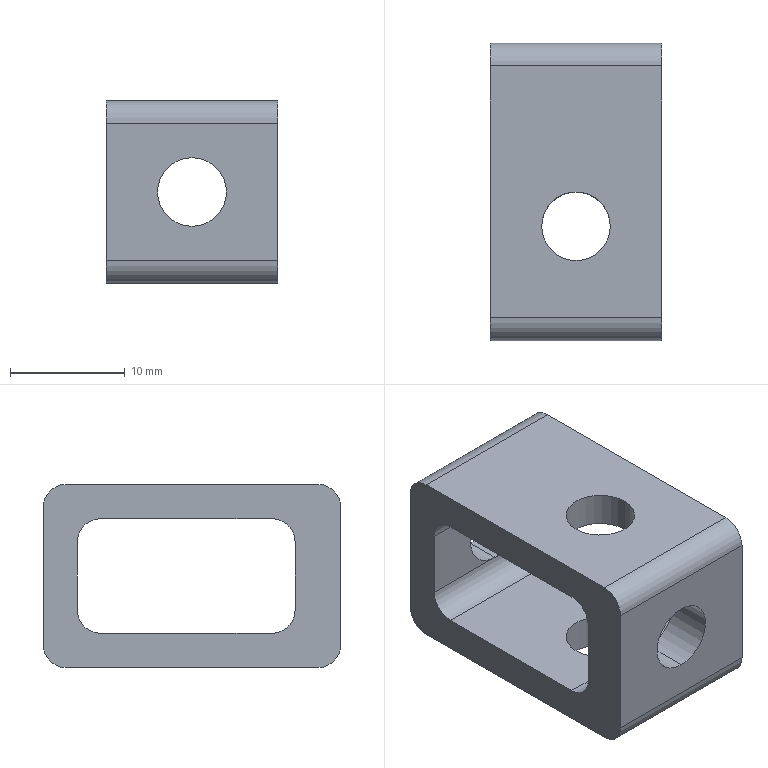Part | SolidWorks | features ICE 3, Fillet 2, Extrusion 1 | 1 solid | 28 faces | box 15 x 26 x 16 mm | volume 3022 mm3 | cylinder 16 | plane 12 | commonest cylinder face diameters 4 x8 6 x8
STEP:
#1=CARTESIAN_POINT('',(0.,-10.,3.));
#2=VERTEX_POINT('',#1);
#3=CARTESIAN_POINT('',(0.,-10.,-3.));
#4=VERTEX_POINT('',#3);
#5=CARTESIAN_POINT('',(0.,-10.,0.));
#6=DIRECTION('',(0.,-1.,0.));
#7=DIRECTION('',(0.,0.,-1.));
#8=AXIS2_PLACEMENT_3D('',#5,#6,#7);
#9=CIRCLE('',#8,3.);
#10=EDGE_CURVE('',#2,#4,#9,.T.);
#11=ORIENTED_EDGE('',*,*,#10,.T.);
#12=CARTESIAN_POINT('',(0.,-6.,-3.));
#13=VERTEX_POINT('',#12);
#14=CARTESIAN_POINT('',(0.,-10.,-3.));
#15=DIRECTION('',(0.,1.,0.));
#16=VECTOR('',#15,1000.);
#17=LINE('',#14,#16);
#18=EDGE_CURVE('',#4,#13,#17,.T.);
#19=ORIENTED_EDGE('',*,*,#18,.T.);
#20=CARTESIAN_POINT('',(0.,-6.,3.));
#21=VERTEX_POINT('',#20);
#22=CARTESIAN_POINT('',(0.,-6.,0.));
#23=DIRECTION('',(0.,-1.,0.));
#24=DIRECTION('',(0.,0.,-1.));
#25=AXIS2_PLACEMENT_3D('',#22,#23,#24);
#26=CIRCLE('',#25,3.);
#27=EDGE_CURVE('',#21,#13,#26,.T.);
#28=ORIENTED_EDGE('',*,*,#27,.F.);
#29=CARTESIAN_POINT('',(0.,-10.,3.));
#30=DIRECTION('',(0.,1.,0.));
#31=VECTOR('',#30,1000.);
#32=LINE('',#29,#31);
#33=EDGE_CURVE('',#2,#21,#32,.T.);
#34=ORIENTED_EDGE('',*,*,#33,.F.);
#35=EDGE_LOOP('',(#11,#19,#28,#34));
#36=FACE_OUTER_BOUND('',#35,.T.);
#37=CARTESIAN_POINT('',(0.,-10.,0.));
#38=DIRECTION('',(0.,1.,0.));
#39=DIRECTION('',(0.,0.,1.));
#40=AXIS2_PLACEMENT_3D('',#37,#38,#39);
#41=CYLINDRICAL_SURFACE('',#40,3.);
#42=ADVANCED_FACE('',(#36),#41,.F.);
#43=CARTESIAN_POINT('',(0.,13.,-3.));
#44=VERTEX_POINT('',#43);
#45=CARTESIAN_POINT('',(0.,13.,3.));
#46=VERTEX_POINT('',#45);
#47=CARTESIAN_POINT('',(0.,13.,0.));
#48=DIRECTION('',(0.,1.,0.));
#49=DIRECTION('',(0.,0.,1.));
#50=AXIS2_PLACEMENT_3D('',#47,#48,#49);
#51=CIRCLE('',#50,3.);
#52=EDGE_CURVE('',#44,#46,#51,.T.);
#53=ORIENTED_EDGE('',*,*,#52,.F.);
#54=CARTESIAN_POINT('',(0.,16.,-3.));
#55=VERTEX_POINT('',#54);
#56=CARTESIAN_POINT('',(0.,-2.,-3.));
#57=DIRECTION('',(0.,1.,0.));
#58=VECTOR('',#57,1000.);
#59=LINE('',#56,#58);
#60=EDGE_CURVE('',#44,#55,#59,.T.);
#61=ORIENTED_EDGE('',*,*,#60,.T.);
#62=CARTESIAN_POINT('',(0.,16.,3.));
#63=VERTEX_POINT('',#62);
#64=CARTESIAN_POINT('',(0.,16.,0.));
#65=DIRECTION('',(0.,1.,0.));
#66=DIRECTION('',(0.,0.,1.));
#67=AXIS2_PLACEMENT_3D('',#64,#65,#66);
#68=CIRCLE('',#67,3.);
#69=EDGE_CURVE('',#55,#63,#68,.T.);
#70=ORIENTED_EDGE('',*,*,#69,.T.);
#71=CARTESIAN_POINT('',(0.,-2.,3.));
#72=DIRECTION('',(0.,1.,0.));
#73=VECTOR('',#72,1000.);
#74=LINE('',#71,#73);
#75=EDGE_CURVE('',#46,#63,#74,.T.);
#76=ORIENTED_EDGE('',*,*,#75,.F.);
#77=EDGE_LOOP('',(#53,#61,#70,#76));
#78=FACE_OUTER_BOUND('',#77,.T.);
#79=CARTESIAN_POINT('',(0.,-2.,0.));
#80=DIRECTION('',(0.,1.,0.));
#81=DIRECTION('',(0.,0.,1.));
#82=AXIS2_PLACEMENT_3D('',#79,#80,#81);
#83=CYLINDRICAL_SURFACE('',#82,3.);
#84=ADVANCED_FACE('',(#78),#83,.F.);
#85=CARTESIAN_POINT('',(3.,0.,-5.));
#86=VERTEX_POINT('',#85);
#87=CARTESIAN_POINT('',(-3.,0.,-5.));
#88=VERTEX_POINT('',#87);
#89=CARTESIAN_POINT('',(0.,0.,-5.));
#90=DIRECTION('',(0.,0.,-1.));
#91=DIRECTION('',(-1.,0.,0.));
#92=AXIS2_PLACEMENT_3D('',#89,#90,#91);
#93=CIRCLE('',#92,3.);
#94=EDGE_CURVE('',#86,#88,#93,.T.);
#95=ORIENTED_EDGE('',*,*,#94,.F.);
#96=CARTESIAN_POINT('',(3.,0.,-8.));
#97=VERTEX_POINT('',#96);
#98=CARTESIAN_POINT('',(3.,0.,8.));
#99=DIRECTION('',(0.,0.,-1.));
#100=VECTOR('',#99,1000.);
#101=LINE('',#98,#100);
#102=EDGE_CURVE('',#86,#97,#101,.T.);
#103=ORIENTED_EDGE('',*,*,#102,.T.);
#104=CARTESIAN_POINT('',(-3.,0.,-8.));
#105=VERTEX_POINT('',#104);
#106=CARTESIAN_POINT('',(0.,0.,-8.));
#107=DIRECTION('',(0.,0.,1.));
#108=DIRECTION('',(1.,0.,0.));
#109=AXIS2_PLACEMENT_3D('',#106,#107,#108);
#110=CIRCLE('',#109,3.);
#111=EDGE_CURVE('',#105,#97,#110,.T.);
#112=ORIENTED_EDGE('',*,*,#111,.F.);
#113=CARTESIAN_POINT('',(-3.,0.,8.));
#114=DIRECTION('',(0.,0.,-1.));
#115=VECTOR('',#114,1000.);
#116=LINE('',#113,#115);
#117=EDGE_CURVE('',#88,#105,#116,.T.);
#118=ORIENTED_EDGE('',*,*,#117,.F.);
#119=EDGE_LOOP('',(#95,#103,#112,#118));
#120=FACE_OUTER_BOUND('',#119,.T.);
#121=CARTESIAN_POINT('',(0.,0.,8.));
#122=DIRECTION('',(0.,0.,-1.));
#123=DIRECTION('',(-1.,0.,0.));
#124=AXIS2_PLACEMENT_3D('',#121,#122,#123);
#125=CYLINDRICAL_SURFACE('',#124,3.);
#126=ADVANCED_FACE('',(#120),#125,.F.);
#127=CARTESIAN_POINT('',(-3.,0.,8.));
#128=VERTEX_POINT('',#127);
#129=CARTESIAN_POINT('',(3.,0.,8.));
#130=VERTEX_POINT('',#129);
#131=CARTESIAN_POINT('',(0.,0.,8.));
#132=DIRECTION('',(0.,0.,1.));
#133=DIRECTION('',(1.,0.,0.));
#134=AXIS2_PLACEMENT_3D('',#131,#132,#133);
#135=CIRCLE('',#134,3.);
#136=EDGE_CURVE('',#128,#130,#135,.T.);
#137=ORIENTED_EDGE('',*,*,#136,.T.);
#138=CARTESIAN_POINT('',(3.,0.,5.));
#139=VERTEX_POINT('',#138);
#140=CARTESIAN_POINT('',(3.,0.,8.));
#141=DIRECTION('',(0.,0.,-1.));
#142=VECTOR('',#141,1000.);
#143=LINE('',#140,#142);
#144=EDGE_CURVE('',#130,#139,#143,.T.);
#145=ORIENTED_EDGE('',*,*,#144,.T.);
#146=CARTESIAN_POINT('',(-3.,0.,5.));
#147=VERTEX_POINT('',#146);
#148=CARTESIAN_POINT('',(0.,0.,5.));
#149=DIRECTION('',(0.,0.,1.));
#150=DIRECTION('',(1.,0.,0.));
#151=AXIS2_PLACEMENT_3D('',#148,#149,#150);
#152=CIRCLE('',#151,3.);
#153=EDGE_CURVE('',#147,#139,#152,.T.);
#154=ORIENTED_EDGE('',*,*,#153,.F.);
#155=CARTESIAN_POINT('',(-3.,0.,8.));
#156=DIRECTION('',(0.,0.,-1.));
#157=VECTOR('',#156,1000.);
#158=LINE('',#155,#157);
#159=EDGE_CURVE('',#128,#147,#158,.T.);
#160=ORIENTED_EDGE('',*,*,#159,.F.);
#161=EDGE_LOOP('',(#137,#145,#154,#160));
#162=FACE_OUTER_BOUND('',#161,.T.);
#163=CARTESIAN_POINT('',(0.,0.,8.));
#164=DIRECTION('',(0.,0.,-1.));
#165=DIRECTION('',(-1.,0.,0.));
#166=AXIS2_PLACEMENT_3D('',#163,#164,#165);
#167=CYLINDRICAL_SURFACE('',#166,3.);
#168=ADVANCED_FACE('',(#162),#167,.F.);
#169=CARTESIAN_POINT('',(7.5,-6.,-3.));
#170=VERTEX_POINT('',#169);
#171=CARTESIAN_POINT('',(7.5,-6.,3.));
#172=VERTEX_POINT('',#171);
#173=CARTESIAN_POINT('',(7.5,-6.,-8.));
#174=DIRECTION('',(0.,0.,1.));
#175=VECTOR('',#174,1000.);
#176=LINE('',#173,#175);
#177=EDGE_CURVE('',#170,#172,#176,.T.);
#178=ORIENTED_EDGE('',*,*,#177,.F.);
#179=CARTESIAN_POINT('',(0.,-6.,-3.));
#180=DIRECTION('',(-1.,0.,0.));
#181=VECTOR('',#180,1000.);
#182=LINE('',#179,#181);
#183=EDGE_CURVE('',#170,#13,#182,.T.);
#184=ORIENTED_EDGE('',*,*,#183,.T.);
#185=CARTESIAN_POINT('',(0.,-6.,0.));
#186=DIRECTION('',(0.,-1.,0.));
#187=DIRECTION('',(0.,0.,-1.));
#188=AXIS2_PLACEMENT_3D('',#185,#186,#187);
#189=CIRCLE('',#188,3.);
#190=EDGE_CURVE('',#13,#21,#189,.T.);
#191=ORIENTED_EDGE('',*,*,#190,.T.);
#192=CARTESIAN_POINT('',(0.,-6.,3.));
#193=DIRECTION('',(1.,0.,0.));
#194=VECTOR('',#193,1000.);
#195=LINE('',#192,#194);
#196=EDGE_CURVE('',#21,#172,#195,.T.);
#197=ORIENTED_EDGE('',*,*,#196,.T.);
#198=EDGE_LOOP('',(#178,#184,#191,#197));
#199=FACE_OUTER_BOUND('',#198,.T.);
#200=CARTESIAN_POINT('',(0.,-6.,0.));
#201=DIRECTION('',(0.,1.,0.));
#202=DIRECTION('',(0.,0.,1.));
#203=AXIS2_PLACEMENT_3D('',#200,#201,#202);
#204=PLANE('',#203);
#205=ADVANCED_FACE('',(#199),#204,.T.);
#206=CARTESIAN_POINT('',(7.5,13.,3.));
#207=VERTEX_POINT('',#206);
#208=CARTESIAN_POINT('',(-7.5,13.,3.));
#209=DIRECTION('',(-1.,0.,0.));
#210=VECTOR('',#209,1000.);
#211=LINE('',#208,#210);
#212=EDGE_CURVE('',#207,#46,#211,.T.);
#213=ORIENTED_EDGE('',*,*,#212,.T.);
#214=CARTESIAN_POINT('',(0.,13.,0.));
#215=DIRECTION('',(0.,1.,0.));
#216=DIRECTION('',(0.,0.,1.));
#217=AXIS2_PLACEMENT_3D('',#214,#215,#216);
#218=CIRCLE('',#217,3.);
#219=EDGE_CURVE('',#46,#44,#218,.T.);
#220=ORIENTED_EDGE('',*,*,#219,.T.);
#221=CARTESIAN_POINT('',(7.5,13.,-3.));
#222=VERTEX_POINT('',#221);
#223=CARTESIAN_POINT('',(7.5,13.,-3.));
#224=DIRECTION('',(1.,0.,0.));
#225=VECTOR('',#224,1000.);
#226=LINE('',#223,#225);
#227=EDGE_CURVE('',#44,#222,#226,.T.);
#228=ORIENTED_EDGE('',*,*,#227,.T.);
#229=CARTESIAN_POINT('',(7.5,13.,5.));
#230=DIRECTION('',(0.,0.,1.));
#231=VECTOR('',#230,1000.);
#232=LINE('',#229,#231);
#233=EDGE_CURVE('',#222,#207,#232,.T.);
#234=ORIENTED_EDGE('',*,*,#233,.T.);
#235=EDGE_LOOP('',(#213,#220,#228,#234));
#236=FACE_OUTER_BOUND('',#235,.T.);
#237=CARTESIAN_POINT('',(-7.5,13.,5.));
#238=DIRECTION('',(0.,1.,0.));
#239=DIRECTION('',(0.,0.,1.));
#240=AXIS2_PLACEMENT_3D('',#237,#238,#239);
#241=PLANE('',#240);
#242=ADVANCED_FACE('',(#236),#241,.F.);
#243=ORIENTED_EDGE('',*,*,#144,.F.);
#244=CARTESIAN_POINT('',(0.,0.,8.));
#245=DIRECTION('',(0.,0.,1.));
#246=DIRECTION('',(1.,0.,0.));
#247=AXIS2_PLACEMENT_3D('',#244,#245,#246);
#248=CIRCLE('',#247,3.);
#249=EDGE_CURVE('',#130,#128,#248,.T.);
#250=ORIENTED_EDGE('',*,*,#249,.T.);
#251=ORIENTED_EDGE('',*,*,#159,.T.);
#252=CARTESIAN_POINT('',(0.,0.,5.));
#253=DIRECTION('',(0.,0.,1.));
#254=DIRECTION('',(1.,0.,0.));
#255=AXIS2_PLACEMENT_3D('',#252,#253,#254);
#256=CIRCLE('',#255,3.);
#257=EDGE_CURVE('',#139,#147,#256,.T.);
#258=ORIENTED_EDGE('',*,*,#257,.F.);
#259=EDGE_LOOP('',(#243,#250,#251,#258));
#260=FACE_OUTER_BOUND('',#259,.T.);
#261=CARTESIAN_POINT('',(0.,0.,8.));
#262=DIRECTION('',(0.,0.,-1.));
#263=DIRECTION('',(-1.,0.,0.));
#264=AXIS2_PLACEMENT_3D('',#261,#262,#263);
#265=CYLINDRICAL_SURFACE('',#264,3.);
#266=ADVANCED_FACE('',(#260),#265,.F.);
#267=CARTESIAN_POINT('',(-7.5,14.,8.));
#268=VERTEX_POINT('',#267);
#269=CARTESIAN_POINT('',(-7.5,-8.,8.));
#270=VERTEX_POINT('',#269);
#271=CARTESIAN_POINT('',(-7.5,-6.,8.));
#272=DIRECTION('',(0.,-1.,0.));
#273=VECTOR('',#272,1000.);
#274=LINE('',#271,#273);
#275=EDGE_CURVE('',#268,#270,#274,.T.);
#276=ORIENTED_EDGE('',*,*,#275,.T.);
#277=CARTESIAN_POINT('',(7.5,-8.,8.));
#278=VERTEX_POINT('',#277);
#279=CARTESIAN_POINT('',(0.,-8.,8.));
#280=DIRECTION('',(1.,0.,0.));
#281=VECTOR('',#280,1000.);
#282=LINE('',#279,#281);
#283=EDGE_CURVE('',#270,#278,#282,.T.);
#284=ORIENTED_EDGE('',*,*,#283,.T.);
#285=CARTESIAN_POINT('',(7.5,14.,8.));
#286=VERTEX_POINT('',#285);
#287=CARTESIAN_POINT('',(7.5,-6.,8.));
#288=DIRECTION('',(0.,1.,0.));
#289=VECTOR('',#288,1000.);
#290=LINE('',#287,#289);
#291=EDGE_CURVE('',#278,#286,#290,.T.);
#292=ORIENTED_EDGE('',*,*,#291,.T.);
#293=CARTESIAN_POINT('',(0.,14.,8.));
#294=DIRECTION('',(-1.,0.,0.));
#295=VECTOR('',#294,1000.);
#296=LINE('',#293,#295);
#297=EDGE_CURVE('',#286,#268,#296,.T.);
#298=ORIENTED_EDGE('',*,*,#297,.T.);
#299=EDGE_LOOP('',(#276,#284,#292,#298));
#300=FACE_OUTER_BOUND('',#299,.T.);
#301=ORIENTED_EDGE('',*,*,#136,.F.);
#302=ORIENTED_EDGE('',*,*,#249,.F.);
#303=EDGE_LOOP('',(#301,#302));
#304=FACE_BOUND('',#303,.T.);
#305=CARTESIAN_POINT('',(0.,0.,8.));
#306=DIRECTION('',(0.,0.,-1.));
#307=DIRECTION('',(-1.,0.,0.));
#308=AXIS2_PLACEMENT_3D('',#305,#306,#307);
#309=PLANE('',#308);
#310=ADVANCED_FACE('',(#300,#304),#309,.F.);
#311=CARTESIAN_POINT('',(7.5,-8.,-8.));
#312=VERTEX_POINT('',#311);
#313=CARTESIAN_POINT('',(7.5,14.,-8.));
#314=VERTEX_POINT('',#313);
#315=CARTESIAN_POINT('',(7.5,-6.,-8.));
#316=DIRECTION('',(0.,1.,0.));
#317=VECTOR('',#316,1000.);
#318=LINE('',#315,#317);
#319=EDGE_CURVE('',#312,#314,#318,.T.);
#320=ORIENTED_EDGE('',*,*,#319,.F.);
#321=CARTESIAN_POINT('',(-7.5,-8.,-8.));
#322=VERTEX_POINT('',#321);
#323=CARTESIAN_POINT('',(-7.5,-8.,-8.));
#324=DIRECTION('',(-1.,0.,0.));
#325=VECTOR('',#324,1000.);
#326=LINE('',#323,#325);
#327=EDGE_CURVE('',#312,#322,#326,.T.);
#328=ORIENTED_EDGE('',*,*,#327,.T.);
#329=CARTESIAN_POINT('',(-7.5,14.,-8.));
#330=VERTEX_POINT('',#329);
#331=CARTESIAN_POINT('',(-7.5,-6.,-8.));
#332=DIRECTION('',(0.,-1.,0.));
#333=VECTOR('',#332,1000.);
#334=LINE('',#331,#333);
#335=EDGE_CURVE('',#330,#322,#334,.T.);
#336=ORIENTED_EDGE('',*,*,#335,.F.);
#337=CARTESIAN_POINT('',(7.5,14.,-8.));
#338=DIRECTION('',(1.,0.,0.));
#339=VECTOR('',#338,1000.);
#340=LINE('',#337,#339);
#341=EDGE_CURVE('',#330,#314,#340,.T.);
#342=ORIENTED_EDGE('',*,*,#341,.T.);
#343=EDGE_LOOP('',(#320,#328,#336,#342));
#344=FACE_OUTER_BOUND('',#343,.T.);
#345=ORIENTED_EDGE('',*,*,#111,.T.);
#346=CARTESIAN_POINT('',(0.,0.,-8.));
#347=DIRECTION('',(0.,0.,1.));
#348=DIRECTION('',(1.,0.,0.));
#349=AXIS2_PLACEMENT_3D('',#346,#347,#348);
#350=CIRCLE('',#349,3.);
#351=EDGE_CURVE('',#97,#105,#350,.T.);
#352=ORIENTED_EDGE('',*,*,#351,.T.);
#353=EDGE_LOOP('',(#345,#352));
#354=FACE_BOUND('',#353,.T.);
#355=CARTESIAN_POINT('',(0.,0.,-8.));
#356=DIRECTION('',(0.,0.,-1.));
#357=DIRECTION('',(-1.,0.,0.));
#358=AXIS2_PLACEMENT_3D('',#355,#356,#357);
#359=PLANE('',#358);
#360=ADVANCED_FACE('',(#344,#354),#359,.T.);
#361=CARTESIAN_POINT('',(-7.5,11.,5.));
#362=VERTEX_POINT('',#361);
#363=CARTESIAN_POINT('',(-7.5,-4.,5.));
#364=VERTEX_POINT('',#363);
#365=CARTESIAN_POINT('',(-7.5,-6.,5.));
#366=DIRECTION('',(0.,-1.,0.));
#367=VECTOR('',#366,1000.);
#368=LINE('',#365,#367);
#369=EDGE_CURVE('',#362,#364,#368,.T.);
#370=ORIENTED_EDGE('',*,*,#369,.T.);
#371=CARTESIAN_POINT('',(-7.5,-6.,3.));
#372=VERTEX_POINT('',#371);
#373=CARTESIAN_POINT('',(-7.5,-4.,3.));
#374=DIRECTION('',(1.,0.,0.));
#375=DIRECTION('',(0.,0.,-1.));
#376=AXIS2_PLACEMENT_3D('',#373,#374,#375);
#377=CIRCLE('',#376,2.);
#378=EDGE_CURVE('',#364,#372,#377,.T.);
#379=ORIENTED_EDGE('',*,*,#378,.T.);
#380=CARTESIAN_POINT('',(-7.5,-6.,-3.));
#381=VERTEX_POINT('',#380);
#382=CARTESIAN_POINT('',(-7.5,-6.,-8.));
#383=DIRECTION('',(0.,0.,-1.));
#384=VECTOR('',#383,1000.);
#385=LINE('',#382,#384);
#386=EDGE_CURVE('',#372,#381,#385,.T.);
#387=ORIENTED_EDGE('',*,*,#386,.T.);
#388=CARTESIAN_POINT('',(-7.5,-4.,-5.));
#389=VERTEX_POINT('',#388);
#390=CARTESIAN_POINT('',(-7.5,-4.,-3.));
#391=DIRECTION('',(1.,0.,0.));
#392=DIRECTION('',(0.,0.,-1.));
#393=AXIS2_PLACEMENT_3D('',#390,#391,#392);
#394=CIRCLE('',#393,2.);
#395=EDGE_CURVE('',#381,#389,#394,.T.);
#396=ORIENTED_EDGE('',*,*,#395,.T.);
#397=CARTESIAN_POINT('',(-7.5,11.,-5.));
#398=VERTEX_POINT('',#397);
#399=CARTESIAN_POINT('',(-7.5,-6.,-5.));
#400=DIRECTION('',(0.,1.,0.));
#401=VECTOR('',#400,1000.);
#402=LINE('',#399,#401);
#403=EDGE_CURVE('',#389,#398,#402,.T.);
#404=ORIENTED_EDGE('',*,*,#403,.T.);
#405=CARTESIAN_POINT('',(-7.5,13.,-3.));
#406=VERTEX_POINT('',#405);
#407=CARTESIAN_POINT('',(-7.5,11.,-3.));
#408=DIRECTION('',(1.,0.,0.));
#409=DIRECTION('',(0.,0.,-1.));
#410=AXIS2_PLACEMENT_3D('',#407,#408,#409);
#411=CIRCLE('',#410,2.);
#412=EDGE_CURVE('',#398,#406,#411,.T.);
#413=ORIENTED_EDGE('',*,*,#412,.T.);
#414=CARTESIAN_POINT('',(-7.5,13.,3.));
#415=VERTEX_POINT('',#414);
#416=CARTESIAN_POINT('',(-7.5,13.,5.));
#417=DIRECTION('',(0.,0.,1.));
#418=VECTOR('',#417,1000.);
#419=LINE('',#416,#418);
#420=EDGE_CURVE('',#406,#415,#419,.T.);
#421=ORIENTED_EDGE('',*,*,#420,.T.);
#422=CARTESIAN_POINT('',(-7.5,11.,3.));
#423=DIRECTION('',(1.,0.,0.));
#424=DIRECTION('',(0.,0.,-1.));
#425=AXIS2_PLACEMENT_3D('',#422,#423,#424);
#426=CIRCLE('',#425,2.);
#427=EDGE_CURVE('',#415,#362,#426,.T.);
#428=ORIENTED_EDGE('',*,*,#427,.T.);
#429=EDGE_LOOP('',(#370,#379,#387,#396,#404,#413,#421,#428));
#430=FACE_BOUND('',#429,.T.);
#431=ORIENTED_EDGE('',*,*,#335,.T.);
#432=CARTESIAN_POINT('',(-7.5,-10.,-6.));
#433=VERTEX_POINT('',#432);
#434=CARTESIAN_POINT('',(-7.5,-8.,-6.));
#435=DIRECTION('',(-1.,0.,0.));
#436=DIRECTION('',(0.,0.,-1.));
#437=AXIS2_PLACEMENT_3D('',#434,#435,#436);
#438=CIRCLE('',#437,2.);
#439=EDGE_CURVE('',#322,#433,#438,.T.);
#440=ORIENTED_EDGE('',*,*,#439,.T.);
#441=CARTESIAN_POINT('',(-7.5,-10.,6.));
#442=VERTEX_POINT('',#441);
#443=CARTESIAN_POINT('',(-7.5,-10.,-8.));
#444=DIRECTION('',(0.,0.,-1.));
#445=VECTOR('',#444,1000.);
#446=LINE('',#443,#445);
#447=EDGE_CURVE('',#442,#433,#446,.T.);
#448=ORIENTED_EDGE('',*,*,#447,.F.);
#449=CARTESIAN_POINT('',(-7.5,-8.,6.));
#450=DIRECTION('',(-1.,0.,0.));
#451=DIRECTION('',(0.,0.,-1.));
#452=AXIS2_PLACEMENT_3D('',#449,#450,#451);
#453=CIRCLE('',#452,2.);
#454=EDGE_CURVE('',#442,#270,#453,.T.);
#455=ORIENTED_EDGE('',*,*,#454,.T.);
#456=ORIENTED_EDGE('',*,*,#275,.F.);
#457=CARTESIAN_POINT('',(-7.5,16.,6.));
#458=VERTEX_POINT('',#457);
#459=CARTESIAN_POINT('',(-7.5,14.,6.));
#460=DIRECTION('',(-1.,0.,0.));
#461=DIRECTION('',(0.,0.,-1.));
#462=AXIS2_PLACEMENT_3D('',#459,#460,#461);
#463=CIRCLE('',#462,2.);
#464=EDGE_CURVE('',#268,#458,#463,.T.);
#465=ORIENTED_EDGE('',*,*,#464,.T.);
#466=CARTESIAN_POINT('',(-7.5,16.,-6.));
#467=VERTEX_POINT('',#466);
#468=CARTESIAN_POINT('',(-7.5,16.,8.));
#469=DIRECTION('',(0.,0.,-1.));
#470=VECTOR('',#469,1000.);
#471=LINE('',#468,#470);
#472=EDGE_CURVE('',#458,#467,#471,.T.);
#473=ORIENTED_EDGE('',*,*,#472,.T.);
#474=CARTESIAN_POINT('',(-7.5,14.,-6.));
#475=DIRECTION('',(-1.,0.,0.));
#476=DIRECTION('',(0.,0.,-1.));
#477=AXIS2_PLACEMENT_3D('',#474,#475,#476);
#478=CIRCLE('',#477,2.);
#479=EDGE_CURVE('',#467,#330,#478,.T.);
#480=ORIENTED_EDGE('',*,*,#479,.T.);
#481=EDGE_LOOP('',(#431,#440,#448,#455,#456,#465,#473,#480));
#482=FACE_OUTER_BOUND('',#481,.T.);
#483=CARTESIAN_POINT('',(-7.5,-6.,8.));
#484=DIRECTION('',(1.,0.,0.));
#485=DIRECTION('',(0.,0.,-1.));
#486=AXIS2_PLACEMENT_3D('',#483,#484,#485);
#487=PLANE('',#486);
#488=ADVANCED_FACE('',(#430,#482),#487,.F.);
#489=CARTESIAN_POINT('',(7.5,-4.,-5.));
#490=VERTEX_POINT('',#489);
#491=CARTESIAN_POINT('',(7.5,11.,-5.));
#492=VERTEX_POINT('',#491);
#493=CARTESIAN_POINT('',(7.5,-6.,-5.));
#494=DIRECTION('',(0.,1.,0.));
#495=VECTOR('',#494,1000.);
#496=LINE('',#493,#495);
#497=EDGE_CURVE('',#490,#492,#496,.T.);
#498=ORIENTED_EDGE('',*,*,#497,.F.);
#499=CARTESIAN_POINT('',(7.5,-4.,-3.));
#500=DIRECTION('',(-1.,0.,0.));
#501=DIRECTION('',(0.,0.,1.));
#502=AXIS2_PLACEMENT_3D('',#499,#500,#501);
#503=CIRCLE('',#502,2.);
#504=EDGE_CURVE('',#490,#170,#503,.T.);
#505=ORIENTED_EDGE('',*,*,#504,.T.);
#506=ORIENTED_EDGE('',*,*,#177,.T.);
#507=CARTESIAN_POINT('',(7.5,-4.,5.));
#508=VERTEX_POINT('',#507);
#509=CARTESIAN_POINT('',(7.5,-4.,3.));
#510=DIRECTION('',(-1.,0.,0.));
#511=DIRECTION('',(0.,0.,1.));
#512=AXIS2_PLACEMENT_3D('',#509,#510,#511);
#513=CIRCLE('',#512,2.);
#514=EDGE_CURVE('',#172,#508,#513,.T.);
#515=ORIENTED_EDGE('',*,*,#514,.T.);
#516=CARTESIAN_POINT('',(7.5,11.,5.));
#517=VERTEX_POINT('',#516);
#518=CARTESIAN_POINT('',(7.5,-6.,5.));
#519=DIRECTION('',(0.,-1.,0.));
#520=VECTOR('',#519,1000.);
#521=LINE('',#518,#520);
#522=EDGE_CURVE('',#517,#508,#521,.T.);
#523=ORIENTED_EDGE('',*,*,#522,.F.);
#524=CARTESIAN_POINT('',(7.5,11.,3.));
#525=DIRECTION('',(-1.,0.,0.));
#526=DIRECTION('',(0.,0.,1.));
#527=AXIS2_PLACEMENT_3D('',#524,#525,#526);
#528=CIRCLE('',#527,2.);
#529=EDGE_CURVE('',#517,#207,#528,.T.);
#530=ORIENTED_EDGE('',*,*,#529,.T.);
#531=ORIENTED_EDGE('',*,*,#233,.F.);
#532=CARTESIAN_POINT('',(7.5,11.,-3.));
#533=DIRECTION('',(-1.,0.,0.));
#534=DIRECTION('',(0.,0.,1.));
#535=AXIS2_PLACEMENT_3D('',#532,#533,#534);
#536=CIRCLE('',#535,2.);
#537=EDGE_CURVE('',#222,#492,#536,.T.);
#538=ORIENTED_EDGE('',*,*,#537,.T.);
#539=EDGE_LOOP('',(#498,#505,#506,#515,#523,#530,#531,#538));
#540=FACE_BOUND('',#539,.T.);
#541=CARTESIAN_POINT('',(7.5,-10.,-6.));
#542=VERTEX_POINT('',#541);
#543=CARTESIAN_POINT('',(7.5,-10.,6.));
#544=VERTEX_POINT('',#543);
#545=CARTESIAN_POINT('',(7.5,-10.,-8.));
#546=DIRECTION('',(0.,0.,1.));
#547=VECTOR('',#546,1000.);
#548=LINE('',#545,#547);
#549=EDGE_CURVE('',#542,#544,#548,.T.);
#550=ORIENTED_EDGE('',*,*,#549,.F.);
#551=CARTESIAN_POINT('',(7.5,-8.,-6.));
#552=DIRECTION('',(1.,0.,0.));
#553=DIRECTION('',(0.,0.,1.));
#554=AXIS2_PLACEMENT_3D('',#551,#552,#553);
#555=CIRCLE('',#554,2.);
#556=EDGE_CURVE('',#542,#312,#555,.T.);
#557=ORIENTED_EDGE('',*,*,#556,.T.);
#558=ORIENTED_EDGE('',*,*,#319,.T.);
#559=CARTESIAN_POINT('',(7.5,16.,-6.));
#560=VERTEX_POINT('',#559);
#561=CARTESIAN_POINT('',(7.5,14.,-6.));
#562=DIRECTION('',(1.,0.,0.));
#563=DIRECTION('',(0.,0.,1.));
#564=AXIS2_PLACEMENT_3D('',#561,#562,#563);
#565=CIRCLE('',#564,2.);
#566=EDGE_CURVE('',#314,#560,#565,.T.);
#567=ORIENTED_EDGE('',*,*,#566,.T.);
#568=CARTESIAN_POINT('',(7.5,16.,6.));
#569=VERTEX_POINT('',#568);
#570=CARTESIAN_POINT('',(7.5,16.,8.));
#571=DIRECTION('',(0.,0.,-1.));
#572=VECTOR('',#571,1000.);
#573=LINE('',#570,#572);
#574=EDGE_CURVE('',#569,#560,#573,.T.);
#575=ORIENTED_EDGE('',*,*,#574,.F.);
#576=CARTESIAN_POINT('',(7.5,14.,6.));
#577=DIRECTION('',(1.,0.,0.));
#578=DIRECTION('',(0.,0.,1.));
#579=AXIS2_PLACEMENT_3D('',#576,#577,#578);
#580=CIRCLE('',#579,2.);
#581=EDGE_CURVE('',#569,#286,#580,.T.);
#582=ORIENTED_EDGE('',*,*,#581,.T.);
#583=ORIENTED_EDGE('',*,*,#291,.F.);
#584=CARTESIAN_POINT('',(7.5,-8.,6.));
#585=DIRECTION('',(1.,0.,0.));
#586=DIRECTION('',(0.,0.,1.));
#587=AXIS2_PLACEMENT_3D('',#584,#585,#586);
#588=CIRCLE('',#587,2.);
#589=EDGE_CURVE('',#278,#544,#588,.T.);
#590=ORIENTED_EDGE('',*,*,#589,.T.);
#591=EDGE_LOOP('',(#550,#557,#558,#567,#575,#582,#583,#590));
#592=FACE_OUTER_BOUND('',#591,.T.);
#593=CARTESIAN_POINT('',(7.5,-6.,8.));
#594=DIRECTION('',(-1.,0.,0.));
#595=DIRECTION('',(0.,0.,1.));
#596=AXIS2_PLACEMENT_3D('',#593,#594,#595);
#597=PLANE('',#596);
#598=ADVANCED_FACE('',(#540,#592),#597,.F.);
#599=CARTESIAN_POINT('',(0.,16.,0.));
#600=DIRECTION('',(0.,1.,0.));
#601=DIRECTION('',(0.,0.,1.));
#602=AXIS2_PLACEMENT_3D('',#599,#600,#601);
#603=CIRCLE('',#602,3.);
#604=EDGE_CURVE('',#63,#55,#603,.T.);
#605=ORIENTED_EDGE('',*,*,#604,.F.);
#606=ORIENTED_EDGE('',*,*,#69,.F.);
#607=EDGE_LOOP('',(#605,#606));
#608=FACE_BOUND('',#607,.T.);
#609=ORIENTED_EDGE('',*,*,#574,.T.);
#610=CARTESIAN_POINT('',(-7.5,16.,-6.));
#611=DIRECTION('',(-1.,0.,0.));
#612=VECTOR('',#611,1000.);
#613=LINE('',#610,#612);
#614=EDGE_CURVE('',#560,#467,#613,.T.);
#615=ORIENTED_EDGE('',*,*,#614,.T.);
#616=ORIENTED_EDGE('',*,*,#472,.F.);
#617=CARTESIAN_POINT('',(-7.5,16.,6.));
#618=DIRECTION('',(1.,0.,0.));
#619=VECTOR('',#618,1000.);
#620=LINE('',#617,#619);
#621=EDGE_CURVE('',#458,#569,#620,.T.);
#622=ORIENTED_EDGE('',*,*,#621,.T.);
#623=EDGE_LOOP('',(#609,#615,#616,#622));
#624=FACE_OUTER_BOUND('',#623,.T.);
#625=CARTESIAN_POINT('',(-7.5,16.,8.));
#626=DIRECTION('',(0.,-1.,0.));
#627=DIRECTION('',(0.,0.,-1.));
#628=AXIS2_PLACEMENT_3D('',#625,#626,#627);
#629=PLANE('',#628);
#630=ADVANCED_FACE('',(#608,#624),#629,.F.);
#631=ORIENTED_EDGE('',*,*,#102,.F.);
#632=CARTESIAN_POINT('',(0.,0.,-5.));
#633=DIRECTION('',(0.,0.,-1.));
#634=DIRECTION('',(-1.,0.,0.));
#635=AXIS2_PLACEMENT_3D('',#632,#633,#634);
#636=CIRCLE('',#635,3.);
#637=EDGE_CURVE('',#88,#86,#636,.T.);
#638=ORIENTED_EDGE('',*,*,#637,.F.);
#639=ORIENTED_EDGE('',*,*,#117,.T.);
#640=ORIENTED_EDGE('',*,*,#351,.F.);
#641=EDGE_LOOP('',(#631,#638,#639,#640));
#642=FACE_OUTER_BOUND('',#641,.T.);
#643=CARTESIAN_POINT('',(0.,0.,8.));
#644=DIRECTION('',(0.,0.,-1.));
#645=DIRECTION('',(-1.,0.,0.));
#646=AXIS2_PLACEMENT_3D('',#643,#644,#645);
#647=CYLINDRICAL_SURFACE('',#646,3.);
#648=ADVANCED_FACE('',(#642),#647,.F.);
#649=ORIENTED_EDGE('',*,*,#153,.T.);
#650=ORIENTED_EDGE('',*,*,#257,.T.);
#651=EDGE_LOOP('',(#649,#650));
#652=FACE_BOUND('',#651,.T.);
#653=ORIENTED_EDGE('',*,*,#522,.T.);
#654=CARTESIAN_POINT('',(-7.5,-4.,5.));
#655=DIRECTION('',(-1.,0.,0.));
#656=VECTOR('',#655,1000.);
#657=LINE('',#654,#656);
#658=EDGE_CURVE('',#508,#364,#657,.T.);
#659=ORIENTED_EDGE('',*,*,#658,.T.);
#660=ORIENTED_EDGE('',*,*,#369,.F.);
#661=CARTESIAN_POINT('',(7.5,11.,5.));
#662=DIRECTION('',(1.,0.,0.));
#663=VECTOR('',#662,1000.);
#664=LINE('',#661,#663);
#665=EDGE_CURVE('',#362,#517,#664,.T.);
#666=ORIENTED_EDGE('',*,*,#665,.T.);
#667=EDGE_LOOP('',(#653,#659,#660,#666));
#668=FACE_OUTER_BOUND('',#667,.T.);
#669=CARTESIAN_POINT('',(-7.5,-6.,5.));
#670=DIRECTION('',(0.,0.,1.));
#671=DIRECTION('',(1.,0.,0.));
#672=AXIS2_PLACEMENT_3D('',#669,#670,#671);
#673=PLANE('',#672);
#674=ADVANCED_FACE('',(#652,#668),#673,.F.);
#675=CARTESIAN_POINT('',(7.5,13.,-3.));
#676=DIRECTION('',(1.,0.,0.));
#677=VECTOR('',#676,1000.);
#678=LINE('',#675,#677);
#679=EDGE_CURVE('',#406,#44,#678,.T.);
#680=ORIENTED_EDGE('',*,*,#679,.T.);
#681=ORIENTED_EDGE('',*,*,#52,.T.);
#682=CARTESIAN_POINT('',(-7.5,13.,3.));
#683=DIRECTION('',(-1.,0.,0.));
#684=VECTOR('',#683,1000.);
#685=LINE('',#682,#684);
#686=EDGE_CURVE('',#46,#415,#685,.T.);
#687=ORIENTED_EDGE('',*,*,#686,.T.);
#688=ORIENTED_EDGE('',*,*,#420,.F.);
#689=EDGE_LOOP('',(#680,#681,#687,#688));
#690=FACE_OUTER_BOUND('',#689,.T.);
#691=CARTESIAN_POINT('',(-7.5,13.,5.));
#692=DIRECTION('',(0.,1.,0.));
#693=DIRECTION('',(0.,0.,1.));
#694=AXIS2_PLACEMENT_3D('',#691,#692,#693);
#695=PLANE('',#694);
#696=ADVANCED_FACE('',(#690),#695,.F.);
#697=ORIENTED_EDGE('',*,*,#637,.T.);
#698=ORIENTED_EDGE('',*,*,#94,.T.);
#699=EDGE_LOOP('',(#697,#698));
#700=FACE_BOUND('',#699,.T.);
#701=ORIENTED_EDGE('',*,*,#403,.F.);
#702=CARTESIAN_POINT('',(-7.5,-4.,-5.));
#703=DIRECTION('',(1.,0.,0.));
#704=VECTOR('',#703,1000.);
#705=LINE('',#702,#704);
#706=EDGE_CURVE('',#389,#490,#705,.T.);
#707=ORIENTED_EDGE('',*,*,#706,.T.);
#708=ORIENTED_EDGE('',*,*,#497,.T.);
#709=CARTESIAN_POINT('',(-7.5,11.,-5.));
#710=DIRECTION('',(-1.,0.,0.));
#711=VECTOR('',#710,1000.);
#712=LINE('',#709,#711);
#713=EDGE_CURVE('',#492,#398,#712,.T.);
#714=ORIENTED_EDGE('',*,*,#713,.T.);
#715=EDGE_LOOP('',(#701,#707,#708,#714));
#716=FACE_OUTER_BOUND('',#715,.T.);
#717=CARTESIAN_POINT('',(-7.5,-6.,-5.));
#718=DIRECTION('',(0.,0.,-1.));
#719=DIRECTION('',(-1.,0.,0.));
#720=AXIS2_PLACEMENT_3D('',#717,#718,#719);
#721=PLANE('',#720);
#722=ADVANCED_FACE('',(#700,#716),#721,.F.);
#723=ORIENTED_EDGE('',*,*,#412,.F.);
#724=ORIENTED_EDGE('',*,*,#713,.F.);
#725=ORIENTED_EDGE('',*,*,#537,.F.);
#726=ORIENTED_EDGE('',*,*,#227,.F.);
#727=ORIENTED_EDGE('',*,*,#679,.F.);
#728=EDGE_LOOP('',(#723,#724,#725,#726,#727));
#729=FACE_OUTER_BOUND('',#728,.T.);
#730=CARTESIAN_POINT('',(-7.5,11.,-3.));
#731=DIRECTION('',(-1.,0.,0.));
#732=DIRECTION('',(0.,0.,1.));
#733=AXIS2_PLACEMENT_3D('',#730,#731,#732);
#734=CYLINDRICAL_SURFACE('',#733,2.);
#735=ADVANCED_FACE('',(#729),#734,.F.);
#736=ORIENTED_EDGE('',*,*,#566,.F.);
#737=ORIENTED_EDGE('',*,*,#341,.F.);
#738=ORIENTED_EDGE('',*,*,#479,.F.);
#739=ORIENTED_EDGE('',*,*,#614,.F.);
#740=EDGE_LOOP('',(#736,#737,#738,#739));
#741=FACE_OUTER_BOUND('',#740,.T.);
#742=CARTESIAN_POINT('',(-7.5,14.,-6.));
#743=DIRECTION('',(1.,0.,0.));
#744=DIRECTION('',(0.,0.,-1.));
#745=AXIS2_PLACEMENT_3D('',#742,#743,#744);
#746=CYLINDRICAL_SURFACE('',#745,2.);
#747=ADVANCED_FACE('',(#741),#746,.T.);
#748=ORIENTED_EDGE('',*,*,#581,.F.);
#749=ORIENTED_EDGE('',*,*,#621,.F.);
#750=ORIENTED_EDGE('',*,*,#464,.F.);
#751=ORIENTED_EDGE('',*,*,#297,.F.);
#752=EDGE_LOOP('',(#748,#749,#750,#751));
#753=FACE_OUTER_BOUND('',#752,.T.);
#754=CARTESIAN_POINT('',(0.,14.,6.));
#755=DIRECTION('',(-1.,0.,0.));
#756=DIRECTION('',(0.,0.,1.));
#757=AXIS2_PLACEMENT_3D('',#754,#755,#756);
#758=CYLINDRICAL_SURFACE('',#757,2.);
#759=ADVANCED_FACE('',(#753),#758,.T.);
#760=ORIENTED_EDGE('',*,*,#427,.F.);
#761=ORIENTED_EDGE('',*,*,#686,.F.);
#762=ORIENTED_EDGE('',*,*,#212,.F.);
#763=ORIENTED_EDGE('',*,*,#529,.F.);
#764=ORIENTED_EDGE('',*,*,#665,.F.);
#765=EDGE_LOOP('',(#760,#761,#762,#763,#764));
#766=FACE_OUTER_BOUND('',#765,.T.);
#767=CARTESIAN_POINT('',(-7.5,11.,3.));
#768=DIRECTION('',(-1.,0.,0.));
#769=DIRECTION('',(0.,0.,1.));
#770=AXIS2_PLACEMENT_3D('',#767,#768,#769);
#771=CYLINDRICAL_SURFACE('',#770,2.);
#772=ADVANCED_FACE('',(#766),#771,.F.);
#773=ORIENTED_EDGE('',*,*,#60,.F.);
#774=ORIENTED_EDGE('',*,*,#219,.F.);
#775=ORIENTED_EDGE('',*,*,#75,.T.);
#776=ORIENTED_EDGE('',*,*,#604,.T.);
#777=EDGE_LOOP('',(#773,#774,#775,#776));
#778=FACE_OUTER_BOUND('',#777,.T.);
#779=CARTESIAN_POINT('',(0.,-2.,0.));
#780=DIRECTION('',(0.,1.,0.));
#781=DIRECTION('',(0.,0.,1.));
#782=AXIS2_PLACEMENT_3D('',#779,#780,#781);
#783=CYLINDRICAL_SURFACE('',#782,3.);
#784=ADVANCED_FACE('',(#778),#783,.F.);
#785=ORIENTED_EDGE('',*,*,#27,.T.);
#786=CARTESIAN_POINT('',(0.,-6.,-3.));
#787=DIRECTION('',(-1.,0.,0.));
#788=VECTOR('',#787,1000.);
#789=LINE('',#786,#788);
#790=EDGE_CURVE('',#13,#381,#789,.T.);
#791=ORIENTED_EDGE('',*,*,#790,.T.);
#792=ORIENTED_EDGE('',*,*,#386,.F.);
#793=CARTESIAN_POINT('',(0.,-6.,3.));
#794=DIRECTION('',(1.,0.,0.));
#795=VECTOR('',#794,1000.);
#796=LINE('',#793,#795);
#797=EDGE_CURVE('',#372,#21,#796,.T.);
#798=ORIENTED_EDGE('',*,*,#797,.T.);
#799=EDGE_LOOP('',(#785,#791,#792,#798));
#800=FACE_OUTER_BOUND('',#799,.T.);
#801=CARTESIAN_POINT('',(0.,-6.,0.));
#802=DIRECTION('',(0.,1.,0.));
#803=DIRECTION('',(0.,0.,1.));
#804=AXIS2_PLACEMENT_3D('',#801,#802,#803);
#805=PLANE('',#804);
#806=ADVANCED_FACE('',(#800),#805,.T.);
#807=ORIENTED_EDGE('',*,*,#447,.T.);
#808=CARTESIAN_POINT('',(7.5,-10.,-6.));
#809=DIRECTION('',(1.,0.,0.));
#810=VECTOR('',#809,1000.);
#811=LINE('',#808,#810);
#812=EDGE_CURVE('',#433,#542,#811,.T.);
#813=ORIENTED_EDGE('',*,*,#812,.T.);
#814=ORIENTED_EDGE('',*,*,#549,.T.);
#815=CARTESIAN_POINT('',(0.,-10.,6.));
#816=DIRECTION('',(-1.,0.,0.));
#817=VECTOR('',#816,1000.);
#818=LINE('',#815,#817);
#819=EDGE_CURVE('',#544,#442,#818,.T.);
#820=ORIENTED_EDGE('',*,*,#819,.T.);
#821=EDGE_LOOP('',(#807,#813,#814,#820));
#822=FACE_OUTER_BOUND('',#821,.T.);
#823=ORIENTED_EDGE('',*,*,#10,.F.);
#824=CARTESIAN_POINT('',(0.,-10.,0.));
#825=DIRECTION('',(0.,-1.,0.));
#826=DIRECTION('',(0.,0.,-1.));
#827=AXIS2_PLACEMENT_3D('',#824,#825,#826);
#828=CIRCLE('',#827,3.);
#829=EDGE_CURVE('',#4,#2,#828,.T.);
#830=ORIENTED_EDGE('',*,*,#829,.F.);
#831=EDGE_LOOP('',(#823,#830));
#832=FACE_BOUND('',#831,.T.);
#833=CARTESIAN_POINT('',(0.,-10.,0.));
#834=DIRECTION('',(0.,1.,0.));
#835=DIRECTION('',(0.,0.,1.));
#836=AXIS2_PLACEMENT_3D('',#833,#834,#835);
#837=PLANE('',#836);
#838=ADVANCED_FACE('',(#822,#832),#837,.F.);
#839=ORIENTED_EDGE('',*,*,#18,.F.);
#840=ORIENTED_EDGE('',*,*,#829,.T.);
#841=ORIENTED_EDGE('',*,*,#33,.T.);
#842=ORIENTED_EDGE('',*,*,#190,.F.);
#843=EDGE_LOOP('',(#839,#840,#841,#842));
#844=FACE_OUTER_BOUND('',#843,.T.);
#845=CARTESIAN_POINT('',(0.,-10.,0.));
#846=DIRECTION('',(0.,1.,0.));
#847=DIRECTION('',(0.,0.,1.));
#848=AXIS2_PLACEMENT_3D('',#845,#846,#847);
#849=CYLINDRICAL_SURFACE('',#848,3.);
#850=ADVANCED_FACE('',(#844),#849,.F.);
#851=ORIENTED_EDGE('',*,*,#790,.F.);
#852=ORIENTED_EDGE('',*,*,#183,.F.);
#853=ORIENTED_EDGE('',*,*,#504,.F.);
#854=ORIENTED_EDGE('',*,*,#706,.F.);
#855=ORIENTED_EDGE('',*,*,#395,.F.);
#856=EDGE_LOOP('',(#851,#852,#853,#854,#855));
#857=FACE_OUTER_BOUND('',#856,.T.);
#858=CARTESIAN_POINT('',(-7.5,-4.,-3.));
#859=DIRECTION('',(1.,0.,0.));
#860=DIRECTION('',(0.,0.,-1.));
#861=AXIS2_PLACEMENT_3D('',#858,#859,#860);
#862=CYLINDRICAL_SURFACE('',#861,2.);
#863=ADVANCED_FACE('',(#857),#862,.F.);
#864=ORIENTED_EDGE('',*,*,#439,.F.);
#865=ORIENTED_EDGE('',*,*,#327,.F.);
#866=ORIENTED_EDGE('',*,*,#556,.F.);
#867=ORIENTED_EDGE('',*,*,#812,.F.);
#868=EDGE_LOOP('',(#864,#865,#866,#867));
#869=FACE_OUTER_BOUND('',#868,.T.);
#870=CARTESIAN_POINT('',(0.,-8.,-6.));
#871=DIRECTION('',(-1.,0.,0.));
#872=DIRECTION('',(0.,0.,1.));
#873=AXIS2_PLACEMENT_3D('',#870,#871,#872);
#874=CYLINDRICAL_SURFACE('',#873,2.);
#875=ADVANCED_FACE('',(#869),#874,.T.);
#876=ORIENTED_EDGE('',*,*,#589,.F.);
#877=ORIENTED_EDGE('',*,*,#283,.F.);
#878=ORIENTED_EDGE('',*,*,#454,.F.);
#879=ORIENTED_EDGE('',*,*,#819,.F.);
#880=EDGE_LOOP('',(#876,#877,#878,#879));
#881=FACE_OUTER_BOUND('',#880,.T.);
#882=CARTESIAN_POINT('',(0.,-8.,6.));
#883=DIRECTION('',(-1.,0.,0.));
#884=DIRECTION('',(0.,0.,1.));
#885=AXIS2_PLACEMENT_3D('',#882,#883,#884);
#886=CYLINDRICAL_SURFACE('',#885,2.);
#887=ADVANCED_FACE('',(#881),#886,.T.);
#888=ORIENTED_EDGE('',*,*,#378,.F.);
#889=ORIENTED_EDGE('',*,*,#658,.F.);
#890=ORIENTED_EDGE('',*,*,#514,.F.);
#891=ORIENTED_EDGE('',*,*,#196,.F.);
#892=ORIENTED_EDGE('',*,*,#797,.F.);
#893=EDGE_LOOP('',(#888,#889,#890,#891,#892));
#894=FACE_OUTER_BOUND('',#893,.T.);
#895=CARTESIAN_POINT('',(0.,-4.,3.));
#896=DIRECTION('',(1.,0.,0.));
#897=DIRECTION('',(0.,0.,-1.));
#898=AXIS2_PLACEMENT_3D('',#895,#896,#897);
#899=CYLINDRICAL_SURFACE('',#898,2.);
#900=ADVANCED_FACE('',(#894),#899,.F.);
#901=CLOSED_SHELL('',(#42,#84,#126,#168,#205,#242,#266,#310,#360,#488,#598,#630,#648,#674,#696,#722,#735,#747,#759,#772,#784,#806,#838,#850,#863,#875,#887,#900));
#902=MANIFOLD_SOLID_BREP('',#901);
#903=CARTESIAN_POINT('',(0.,0.,0.));
#904=DIRECTION('',(0.,0.,1.));
#905=DIRECTION('',(1.,0.,0.));
#906=AXIS2_PLACEMENT_3D('',#903,#904,#905);
#907=(LENGTH_UNIT()NAMED_UNIT(*)SI_UNIT(.MILLI.,.METRE.));
#908=UNCERTAINTY_MEASURE_WITH_UNIT(LENGTH_MEASURE(0.00001),#907,'','');
#909=(NAMED_UNIT(*)PLANE_ANGLE_UNIT()SI_UNIT($,.RADIAN.));
#910=(NAMED_UNIT(*)SI_UNIT($,.STERADIAN.)SOLID_ANGLE_UNIT());
#911=(GEOMETRIC_REPRESENTATION_CONTEXT(3)GLOBAL_UNCERTAINTY_ASSIGNED_CONTEXT((#908))GLOBAL_UNIT_ASSIGNED_CONTEXT((#907,#909,#910))REPRESENTATION_CONTEXT('',''));
#912=ADVANCED_BREP_SHAPE_REPRESENTATION('',(#902,#906),#911);